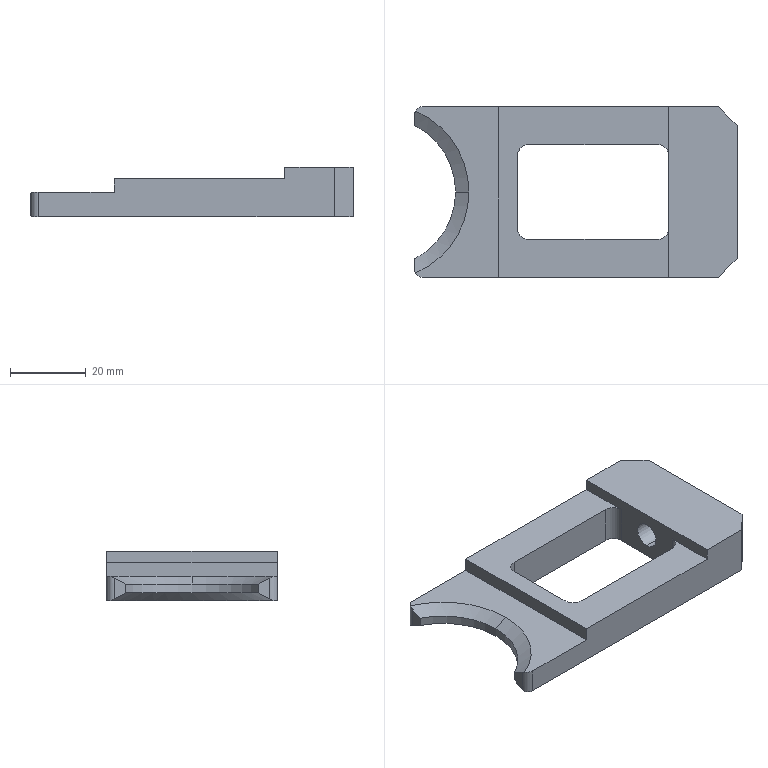Part | SolidWorks | features ICE 6, Chamfer 3, Fillet 3, Extrusion 1, HoleWzd 1 | 1 solid | 28 faces | box 85 x 45 x 13 mm | volume 24143 mm3 | plane 16 | cylinder 9 | cone 3 | commonest cylinder face diameters 6 x4 4 x2 6.8 x2 39.5 x1
STEP:
#1=CARTESIAN_POINT('',(80.,0.,-0.1));
#2=VERTEX_POINT('',#1);
#3=CARTESIAN_POINT('',(80.,0.,-6.9));
#4=VERTEX_POINT('',#3);
#5=CARTESIAN_POINT('',(80.,0.,-3.5));
#6=DIRECTION('',(1.,0.,0.));
#7=DIRECTION('',(0.,0.,-1.));
#8=AXIS2_PLACEMENT_3D('',#5,#6,#7);
#9=CIRCLE('',#8,3.4);
#10=EDGE_CURVE('',#2,#4,#9,.T.);
#11=ORIENTED_EDGE('',*,*,#10,.F.);
#12=CARTESIAN_POINT('',(98.,0.,-0.1));
#13=VERTEX_POINT('',#12);
#14=CARTESIAN_POINT('',(98.,0.,-0.1));
#15=DIRECTION('',(1.,0.,0.));
#16=VECTOR('',#15,1000.);
#17=LINE('',#14,#16);
#18=EDGE_CURVE('',#2,#13,#17,.T.);
#19=ORIENTED_EDGE('',*,*,#18,.T.);
#20=CARTESIAN_POINT('',(98.,0.,-6.9));
#21=VERTEX_POINT('',#20);
#22=CARTESIAN_POINT('',(98.,0.,-3.5));
#23=DIRECTION('',(1.,0.,0.));
#24=DIRECTION('',(0.,0.,-1.));
#25=AXIS2_PLACEMENT_3D('',#22,#23,#24);
#26=CIRCLE('',#25,3.4);
#27=EDGE_CURVE('',#13,#21,#26,.T.);
#28=ORIENTED_EDGE('',*,*,#27,.T.);
#29=CARTESIAN_POINT('',(98.,0.,-6.9));
#30=DIRECTION('',(1.,0.,0.));
#31=VECTOR('',#30,1000.);
#32=LINE('',#29,#31);
#33=EDGE_CURVE('',#4,#21,#32,.T.);
#34=ORIENTED_EDGE('',*,*,#33,.F.);
#35=EDGE_LOOP('',(#11,#19,#28,#34));
#36=FACE_OUTER_BOUND('',#35,.T.);
#37=CARTESIAN_POINT('',(98.,0.,-3.5));
#38=DIRECTION('',(1.,0.,0.));
#39=DIRECTION('',(0.,0.,-1.));
#40=AXIS2_PLACEMENT_3D('',#37,#38,#39);
#41=CYLINDRICAL_SURFACE('',#40,3.4);
#42=ADVANCED_FACE('',(#36),#41,.F.);
#43=CARTESIAN_POINT('',(23.75,0.,-5.62));
#44=VERTEX_POINT('',#43);
#45=CARTESIAN_POINT('',(13.,17.58,-5.62));
#46=VERTEX_POINT('',#45);
#47=CARTESIAN_POINT('',(4.,0.,-5.62));
#48=DIRECTION('',(0.,0.,1.));
#49=DIRECTION('',(-1.,0.,0.));
#50=AXIS2_PLACEMENT_3D('',#47,#48,#49);
#51=CIRCLE('',#50,19.75);
#52=EDGE_CURVE('',#44,#46,#51,.T.);
#53=ORIENTED_EDGE('',*,*,#52,.F.);
#54=CARTESIAN_POINT('',(27.25,0.,-3.6));
#55=VERTEX_POINT('',#54);
#56=CARTESIAN_POINT('',(23.75,0.,-5.62));
#57=DIRECTION('',(0.8661,0.,0.4999));
#58=VECTOR('',#57,1000.);
#59=LINE('',#56,#58);
#60=EDGE_CURVE('',#44,#55,#59,.T.);
#61=ORIENTED_EDGE('',*,*,#60,.T.);
#62=CARTESIAN_POINT('',(13.192,21.356,-3.6));
#63=VERTEX_POINT('',#62);
#64=CARTESIAN_POINT('',(4.,0.,-3.6));
#65=DIRECTION('',(0.,0.,-1.));
#66=DIRECTION('',(-1.,0.,0.));
#67=AXIS2_PLACEMENT_3D('',#64,#65,#66);
#68=CIRCLE('',#67,23.25);
#69=EDGE_CURVE('',#63,#55,#68,.T.);
#70=ORIENTED_EDGE('',*,*,#69,.F.);
#71=CARTESIAN_POINT('',(13.,20.5,-4.097));
#72=VERTEX_POINT('',#71);
#73=CARTESIAN_POINT('',(13.192,21.356,-3.6));
#74=CARTESIAN_POINT('',(13.065,21.088,-3.771));
#75=CARTESIAN_POINT('',(13.,20.803,-3.937));
#76=CARTESIAN_POINT('',(13.,20.5,-4.097));
#77=B_SPLINE_CURVE_WITH_KNOTS('',3,(#73,#74,#75,#76),.UNSPECIFIED.,.F.,.F.,(4,4),(0.,0.001008),.UNSPECIFIED.);
#78=EDGE_CURVE('',#63,#72,#77,.T.);
#79=ORIENTED_EDGE('',*,*,#78,.T.);
#80=CARTESIAN_POINT('',(13.,17.58,-5.62));
#81=CARTESIAN_POINT('',(13.,18.556,-5.119));
#82=CARTESIAN_POINT('',(13.,19.529,-4.61));
#83=CARTESIAN_POINT('',(13.,20.5,-4.097));
#84=B_SPLINE_CURVE_WITH_KNOTS('',3,(#80,#81,#82,#83),.UNSPECIFIED.,.F.,.F.,(4,4),(0.04213,0.04546),.UNSPECIFIED.);
#85=EDGE_CURVE('',#46,#72,#84,.T.);
#86=ORIENTED_EDGE('',*,*,#85,.F.);
#87=EDGE_LOOP('',(#53,#61,#70,#79,#86));
#88=FACE_OUTER_BOUND('',#87,.T.);
#89=CARTESIAN_POINT('',(4.,0.,-5.62));
#90=DIRECTION('',(0.,0.,1.));
#91=DIRECTION('',(1.,0.,0.));
#92=AXIS2_PLACEMENT_3D('',#89,#90,#91);
#93=CONICAL_SURFACE('',#92,19.75,1.047);
#94=ADVANCED_FACE('',(#88),#93,.F.);
#95=CARTESIAN_POINT('',(80.,-9.5,0.));
#96=VERTEX_POINT('',#95);
#97=CARTESIAN_POINT('',(80.,-22.5,0.));
#98=VERTEX_POINT('',#97);
#99=CARTESIAN_POINT('',(80.,22.5,0.));
#100=DIRECTION('',(0.,-1.,0.));
#101=VECTOR('',#100,1000.);
#102=LINE('',#99,#101);
#103=EDGE_CURVE('',#96,#98,#102,.T.);
#104=ORIENTED_EDGE('',*,*,#103,.F.);
#105=CARTESIAN_POINT('',(77.,-12.5,0.));
#106=VERTEX_POINT('',#105);
#107=CARTESIAN_POINT('',(77.,-9.5,0.));
#108=DIRECTION('',(0.,0.,-1.));
#109=DIRECTION('',(-1.,0.,0.));
#110=AXIS2_PLACEMENT_3D('',#107,#108,#109);
#111=CIRCLE('',#110,3.);
#112=EDGE_CURVE('',#96,#106,#111,.T.);
#113=ORIENTED_EDGE('',*,*,#112,.T.);
#114=CARTESIAN_POINT('',(43.,-12.5,0.));
#115=VERTEX_POINT('',#114);
#116=CARTESIAN_POINT('',(40.,-12.5,0.));
#117=DIRECTION('',(1.,0.,0.));
#118=VECTOR('',#117,1000.);
#119=LINE('',#116,#118);
#120=EDGE_CURVE('',#115,#106,#119,.T.);
#121=ORIENTED_EDGE('',*,*,#120,.F.);
#122=CARTESIAN_POINT('',(40.,-9.5,0.));
#123=VERTEX_POINT('',#122);
#124=CARTESIAN_POINT('',(43.,-9.5,0.));
#125=DIRECTION('',(0.,0.,-1.));
#126=DIRECTION('',(-1.,0.,0.));
#127=AXIS2_PLACEMENT_3D('',#124,#125,#126);
#128=CIRCLE('',#127,3.);
#129=EDGE_CURVE('',#115,#123,#128,.T.);
#130=ORIENTED_EDGE('',*,*,#129,.T.);
#131=CARTESIAN_POINT('',(40.,9.5,0.));
#132=VERTEX_POINT('',#131);
#133=CARTESIAN_POINT('',(40.,12.5,0.));
#134=DIRECTION('',(0.,-1.,0.));
#135=VECTOR('',#134,1000.);
#136=LINE('',#133,#135);
#137=EDGE_CURVE('',#132,#123,#136,.T.);
#138=ORIENTED_EDGE('',*,*,#137,.F.);
#139=CARTESIAN_POINT('',(43.,12.5,0.));
#140=VERTEX_POINT('',#139);
#141=CARTESIAN_POINT('',(43.,9.5,0.));
#142=DIRECTION('',(0.,0.,-1.));
#143=DIRECTION('',(-1.,0.,0.));
#144=AXIS2_PLACEMENT_3D('',#141,#142,#143);
#145=CIRCLE('',#144,3.);
#146=EDGE_CURVE('',#132,#140,#145,.T.);
#147=ORIENTED_EDGE('',*,*,#146,.T.);
#148=CARTESIAN_POINT('',(77.,12.5,0.));
#149=VERTEX_POINT('',#148);
#150=CARTESIAN_POINT('',(40.,12.5,0.));
#151=DIRECTION('',(-1.,0.,0.));
#152=VECTOR('',#151,1000.);
#153=LINE('',#150,#152);
#154=EDGE_CURVE('',#149,#140,#153,.T.);
#155=ORIENTED_EDGE('',*,*,#154,.F.);
#156=CARTESIAN_POINT('',(80.,9.5,0.));
#157=VERTEX_POINT('',#156);
#158=CARTESIAN_POINT('',(77.,9.5,0.));
#159=DIRECTION('',(0.,0.,-1.));
#160=DIRECTION('',(-1.,0.,0.));
#161=AXIS2_PLACEMENT_3D('',#158,#159,#160);
#162=CIRCLE('',#161,3.);
#163=EDGE_CURVE('',#149,#157,#162,.T.);
#164=ORIENTED_EDGE('',*,*,#163,.T.);
#165=CARTESIAN_POINT('',(80.,22.5,0.));
#166=VERTEX_POINT('',#165);
#167=CARTESIAN_POINT('',(80.,22.5,0.));
#168=DIRECTION('',(0.,-1.,0.));
#169=VECTOR('',#168,1000.);
#170=LINE('',#167,#169);
#171=EDGE_CURVE('',#166,#157,#170,.T.);
#172=ORIENTED_EDGE('',*,*,#171,.F.);
#173=CARTESIAN_POINT('',(35.,22.5,0.));
#174=VERTEX_POINT('',#173);
#175=CARTESIAN_POINT('',(0.,22.5,0.));
#176=DIRECTION('',(1.,0.,0.));
#177=VECTOR('',#176,1000.);
#178=LINE('',#175,#177);
#179=EDGE_CURVE('',#174,#166,#178,.T.);
#180=ORIENTED_EDGE('',*,*,#179,.F.);
#181=CARTESIAN_POINT('',(35.,-22.5,0.));
#182=VERTEX_POINT('',#181);
#183=CARTESIAN_POINT('',(35.,22.5,0.));
#184=DIRECTION('',(0.,-1.,0.));
#185=VECTOR('',#184,1000.);
#186=LINE('',#183,#185);
#187=EDGE_CURVE('',#174,#182,#186,.T.);
#188=ORIENTED_EDGE('',*,*,#187,.T.);
#189=CARTESIAN_POINT('',(0.,-22.5,0.));
#190=DIRECTION('',(1.,0.,0.));
#191=VECTOR('',#190,1000.);
#192=LINE('',#189,#191);
#193=EDGE_CURVE('',#182,#98,#192,.T.);
#194=ORIENTED_EDGE('',*,*,#193,.T.);
#195=EDGE_LOOP('',(#104,#113,#121,#130,#138,#147,#155,#164,#172,#180,#188,#194));
#196=FACE_OUTER_BOUND('',#195,.T.);
#197=CARTESIAN_POINT('',(0.,22.5,0.));
#198=DIRECTION('',(0.,0.,-1.));
#199=DIRECTION('',(-1.,0.,0.));
#200=AXIS2_PLACEMENT_3D('',#197,#198,#199);
#201=PLANE('',#200);
#202=ADVANCED_FACE('',(#196),#201,.F.);
#203=CARTESIAN_POINT('',(80.,0.,-3.5));
#204=DIRECTION('',(1.,0.,0.));
#205=DIRECTION('',(0.,0.,-1.));
#206=AXIS2_PLACEMENT_3D('',#203,#204,#205);
#207=CIRCLE('',#206,3.4);
#208=EDGE_CURVE('',#4,#2,#207,.T.);
#209=ORIENTED_EDGE('',*,*,#208,.T.);
#210=ORIENTED_EDGE('',*,*,#10,.T.);
#211=EDGE_LOOP('',(#209,#210));
#212=FACE_BOUND('',#211,.T.);
#213=ORIENTED_EDGE('',*,*,#171,.T.);
#214=CARTESIAN_POINT('',(80.,9.5,-10.));
#215=VERTEX_POINT('',#214);
#216=CARTESIAN_POINT('',(80.,9.5,-10.));
#217=DIRECTION('',(0.,0.,-1.));
#218=VECTOR('',#217,1000.);
#219=LINE('',#216,#218);
#220=EDGE_CURVE('',#157,#215,#219,.T.);
#221=ORIENTED_EDGE('',*,*,#220,.T.);
#222=CARTESIAN_POINT('',(80.,-9.5,-10.));
#223=VERTEX_POINT('',#222);
#224=CARTESIAN_POINT('',(80.,22.5,-10.));
#225=DIRECTION('',(0.,1.,0.));
#226=VECTOR('',#225,1000.);
#227=LINE('',#224,#226);
#228=EDGE_CURVE('',#223,#215,#227,.T.);
#229=ORIENTED_EDGE('',*,*,#228,.F.);
#230=CARTESIAN_POINT('',(80.,-9.5,0.));
#231=DIRECTION('',(0.,0.,1.));
#232=VECTOR('',#231,1000.);
#233=LINE('',#230,#232);
#234=EDGE_CURVE('',#223,#96,#233,.T.);
#235=ORIENTED_EDGE('',*,*,#234,.T.);
#236=ORIENTED_EDGE('',*,*,#103,.T.);
#237=CARTESIAN_POINT('',(80.,-22.5,3.));
#238=VERTEX_POINT('',#237);
#239=CARTESIAN_POINT('',(80.,-22.5,0.));
#240=DIRECTION('',(0.,0.,1.));
#241=VECTOR('',#240,1000.);
#242=LINE('',#239,#241);
#243=EDGE_CURVE('',#98,#238,#242,.T.);
#244=ORIENTED_EDGE('',*,*,#243,.T.);
#245=CARTESIAN_POINT('',(80.,22.5,3.));
#246=VERTEX_POINT('',#245);
#247=CARTESIAN_POINT('',(80.,22.5,3.));
#248=DIRECTION('',(0.,-1.,0.));
#249=VECTOR('',#248,1000.);
#250=LINE('',#247,#249);
#251=EDGE_CURVE('',#246,#238,#250,.T.);
#252=ORIENTED_EDGE('',*,*,#251,.F.);
#253=CARTESIAN_POINT('',(80.,22.5,0.));
#254=DIRECTION('',(0.,0.,1.));
#255=VECTOR('',#254,1000.);
#256=LINE('',#253,#255);
#257=EDGE_CURVE('',#166,#246,#256,.T.);
#258=ORIENTED_EDGE('',*,*,#257,.F.);
#259=EDGE_LOOP('',(#213,#221,#229,#235,#236,#244,#252,#258));
#260=FACE_OUTER_BOUND('',#259,.T.);
#261=CARTESIAN_POINT('',(80.,22.5,0.));
#262=DIRECTION('',(1.,0.,0.));
#263=DIRECTION('',(0.,0.,-1.));
#264=AXIS2_PLACEMENT_3D('',#261,#262,#263);
#265=PLANE('',#264);
#266=ADVANCED_FACE('',(#212,#260),#265,.F.);
#267=CARTESIAN_POINT('',(93.,-22.5,3.));
#268=VERTEX_POINT('',#267);
#269=CARTESIAN_POINT('',(80.,-22.5,3.));
#270=DIRECTION('',(1.,0.,0.));
#271=VECTOR('',#270,1000.);
#272=LINE('',#269,#271);
#273=EDGE_CURVE('',#238,#268,#272,.T.);
#274=ORIENTED_EDGE('',*,*,#273,.T.);
#275=CARTESIAN_POINT('',(98.,-17.5,3.));
#276=VERTEX_POINT('',#275);
#277=CARTESIAN_POINT('',(98.,-17.5,3.));
#278=DIRECTION('',(0.7071,0.7071,0.));
#279=VECTOR('',#278,1000.);
#280=LINE('',#277,#279);
#281=EDGE_CURVE('',#268,#276,#280,.T.);
#282=ORIENTED_EDGE('',*,*,#281,.T.);
#283=CARTESIAN_POINT('',(98.,17.5,3.));
#284=VERTEX_POINT('',#283);
#285=CARTESIAN_POINT('',(98.,22.5,3.));
#286=DIRECTION('',(0.,-1.,0.));
#287=VECTOR('',#286,1000.);
#288=LINE('',#285,#287);
#289=EDGE_CURVE('',#284,#276,#288,.T.);
#290=ORIENTED_EDGE('',*,*,#289,.F.);
#291=CARTESIAN_POINT('',(93.,22.5,3.));
#292=VERTEX_POINT('',#291);
#293=CARTESIAN_POINT('',(93.,22.5,3.));
#294=DIRECTION('',(-0.7071,0.7071,0.));
#295=VECTOR('',#294,1000.);
#296=LINE('',#293,#295);
#297=EDGE_CURVE('',#284,#292,#296,.T.);
#298=ORIENTED_EDGE('',*,*,#297,.T.);
#299=CARTESIAN_POINT('',(80.,22.5,3.));
#300=DIRECTION('',(1.,0.,0.));
#301=VECTOR('',#300,1000.);
#302=LINE('',#299,#301);
#303=EDGE_CURVE('',#246,#292,#302,.T.);
#304=ORIENTED_EDGE('',*,*,#303,.F.);
#305=ORIENTED_EDGE('',*,*,#251,.T.);
#306=EDGE_LOOP('',(#274,#282,#290,#298,#304,#305));
#307=FACE_OUTER_BOUND('',#306,.T.);
#308=CARTESIAN_POINT('',(80.,22.5,3.));
#309=DIRECTION('',(0.,0.,-1.));
#310=DIRECTION('',(-1.,0.,0.));
#311=AXIS2_PLACEMENT_3D('',#308,#309,#310);
#312=PLANE('',#311);
#313=ADVANCED_FACE('',(#307),#312,.F.);
#314=CARTESIAN_POINT('',(98.,0.,-3.5));
#315=DIRECTION('',(1.,0.,0.));
#316=DIRECTION('',(0.,0.,-1.));
#317=AXIS2_PLACEMENT_3D('',#314,#315,#316);
#318=CIRCLE('',#317,3.4);
#319=EDGE_CURVE('',#21,#13,#318,.T.);
#320=ORIENTED_EDGE('',*,*,#319,.F.);
#321=ORIENTED_EDGE('',*,*,#27,.F.);
#322=EDGE_LOOP('',(#320,#321));
#323=FACE_BOUND('',#322,.T.);
#324=ORIENTED_EDGE('',*,*,#289,.T.);
#325=CARTESIAN_POINT('',(98.,-17.5,-10.));
#326=VERTEX_POINT('',#325);
#327=CARTESIAN_POINT('',(98.,-17.5,3.));
#328=DIRECTION('',(0.,0.,-1.));
#329=VECTOR('',#328,1000.);
#330=LINE('',#327,#329);
#331=EDGE_CURVE('',#276,#326,#330,.T.);
#332=ORIENTED_EDGE('',*,*,#331,.T.);
#333=CARTESIAN_POINT('',(98.,17.5,-10.));
#334=VERTEX_POINT('',#333);
#335=CARTESIAN_POINT('',(98.,22.5,-10.));
#336=DIRECTION('',(0.,-1.,0.));
#337=VECTOR('',#336,1000.);
#338=LINE('',#335,#337);
#339=EDGE_CURVE('',#334,#326,#338,.T.);
#340=ORIENTED_EDGE('',*,*,#339,.F.);
#341=CARTESIAN_POINT('',(98.,17.5,3.));
#342=DIRECTION('',(0.,0.,1.));
#343=VECTOR('',#342,1000.);
#344=LINE('',#341,#343);
#345=EDGE_CURVE('',#334,#284,#344,.T.);
#346=ORIENTED_EDGE('',*,*,#345,.T.);
#347=EDGE_LOOP('',(#324,#332,#340,#346));
#348=FACE_OUTER_BOUND('',#347,.T.);
#349=CARTESIAN_POINT('',(98.,22.5,3.));
#350=DIRECTION('',(-1.,0.,0.));
#351=DIRECTION('',(0.,0.,1.));
#352=AXIS2_PLACEMENT_3D('',#349,#350,#351);
#353=PLANE('',#352);
#354=ADVANCED_FACE('',(#323,#348),#353,.F.);
#355=CARTESIAN_POINT('',(40.,9.5,-10.));
#356=VERTEX_POINT('',#355);
#357=CARTESIAN_POINT('',(40.,-9.5,-10.));
#358=VERTEX_POINT('',#357);
#359=CARTESIAN_POINT('',(40.,22.5,-10.));
#360=DIRECTION('',(0.,-1.,0.));
#361=VECTOR('',#360,1000.);
#362=LINE('',#359,#361);
#363=EDGE_CURVE('',#356,#358,#362,.T.);
#364=ORIENTED_EDGE('',*,*,#363,.T.);
#365=CARTESIAN_POINT('',(43.,-12.5,-10.));
#366=VERTEX_POINT('',#365);
#367=CARTESIAN_POINT('',(43.,-9.5,-10.));
#368=DIRECTION('',(0.,0.,1.));
#369=DIRECTION('',(1.,0.,0.));
#370=AXIS2_PLACEMENT_3D('',#367,#368,#369);
#371=CIRCLE('',#370,3.);
#372=EDGE_CURVE('',#358,#366,#371,.T.);
#373=ORIENTED_EDGE('',*,*,#372,.T.);
#374=CARTESIAN_POINT('',(77.,-12.5,-10.));
#375=VERTEX_POINT('',#374);
#376=CARTESIAN_POINT('',(98.,-12.5,-10.));
#377=DIRECTION('',(1.,0.,0.));
#378=VECTOR('',#377,1000.);
#379=LINE('',#376,#378);
#380=EDGE_CURVE('',#366,#375,#379,.T.);
#381=ORIENTED_EDGE('',*,*,#380,.T.);
#382=CARTESIAN_POINT('',(77.,-9.5,-10.));
#383=DIRECTION('',(0.,0.,1.));
#384=DIRECTION('',(1.,0.,0.));
#385=AXIS2_PLACEMENT_3D('',#382,#383,#384);
#386=CIRCLE('',#385,3.);
#387=EDGE_CURVE('',#375,#223,#386,.T.);
#388=ORIENTED_EDGE('',*,*,#387,.T.);
#389=ORIENTED_EDGE('',*,*,#228,.T.);
#390=CARTESIAN_POINT('',(77.,12.5,-10.));
#391=VERTEX_POINT('',#390);
#392=CARTESIAN_POINT('',(77.,9.5,-10.));
#393=DIRECTION('',(0.,0.,1.));
#394=DIRECTION('',(1.,0.,0.));
#395=AXIS2_PLACEMENT_3D('',#392,#393,#394);
#396=CIRCLE('',#395,3.);
#397=EDGE_CURVE('',#215,#391,#396,.T.);
#398=ORIENTED_EDGE('',*,*,#397,.T.);
#399=CARTESIAN_POINT('',(43.,12.5,-10.));
#400=VERTEX_POINT('',#399);
#401=CARTESIAN_POINT('',(98.,12.5,-10.));
#402=DIRECTION('',(-1.,0.,0.));
#403=VECTOR('',#402,1000.);
#404=LINE('',#401,#403);
#405=EDGE_CURVE('',#391,#400,#404,.T.);
#406=ORIENTED_EDGE('',*,*,#405,.T.);
#407=CARTESIAN_POINT('',(43.,9.5,-10.));
#408=DIRECTION('',(0.,0.,1.));
#409=DIRECTION('',(1.,0.,0.));
#410=AXIS2_PLACEMENT_3D('',#407,#408,#409);
#411=CIRCLE('',#410,3.);
#412=EDGE_CURVE('',#400,#356,#411,.T.);
#413=ORIENTED_EDGE('',*,*,#412,.T.);
#414=EDGE_LOOP('',(#364,#373,#381,#388,#389,#398,#406,#413));
#415=FACE_BOUND('',#414,.T.);
#416=CARTESIAN_POINT('',(13.192,-21.356,-10.));
#417=VERTEX_POINT('',#416);
#418=CARTESIAN_POINT('',(13.192,21.356,-10.));
#419=VERTEX_POINT('',#418);
#420=CARTESIAN_POINT('',(4.,0.,-10.));
#421=DIRECTION('',(0.,0.,1.));
#422=DIRECTION('',(1.,0.,0.));
#423=AXIS2_PLACEMENT_3D('',#420,#421,#422);
#424=CIRCLE('',#423,23.25);
#425=EDGE_CURVE('',#417,#419,#424,.T.);
#426=ORIENTED_EDGE('',*,*,#425,.T.);
#427=CARTESIAN_POINT('',(15.,22.5,-10.));
#428=VERTEX_POINT('',#427);
#429=CARTESIAN_POINT('',(15.,20.5,-10.));
#430=DIRECTION('',(0.,0.,-1.));
#431=DIRECTION('',(1.,0.,0.));
#432=AXIS2_PLACEMENT_3D('',#429,#430,#431);
#433=CIRCLE('',#432,2.);
#434=EDGE_CURVE('',#419,#428,#433,.T.);
#435=ORIENTED_EDGE('',*,*,#434,.T.);
#436=CARTESIAN_POINT('',(93.,22.5,-10.));
#437=VERTEX_POINT('',#436);
#438=CARTESIAN_POINT('',(98.,22.5,-10.));
#439=DIRECTION('',(-1.,0.,0.));
#440=VECTOR('',#439,1000.);
#441=LINE('',#438,#440);
#442=EDGE_CURVE('',#437,#428,#441,.T.);
#443=ORIENTED_EDGE('',*,*,#442,.F.);
#444=CARTESIAN_POINT('',(93.,22.5,-10.));
#445=DIRECTION('',(0.7071,-0.7071,0.));
#446=VECTOR('',#445,1000.);
#447=LINE('',#444,#446);
#448=EDGE_CURVE('',#437,#334,#447,.T.);
#449=ORIENTED_EDGE('',*,*,#448,.T.);
#450=ORIENTED_EDGE('',*,*,#339,.T.);
#451=CARTESIAN_POINT('',(93.,-22.5,-10.));
#452=VERTEX_POINT('',#451);
#453=CARTESIAN_POINT('',(98.,-17.5,-10.));
#454=DIRECTION('',(-0.7071,-0.7071,0.));
#455=VECTOR('',#454,1000.);
#456=LINE('',#453,#455);
#457=EDGE_CURVE('',#326,#452,#456,.T.);
#458=ORIENTED_EDGE('',*,*,#457,.T.);
#459=CARTESIAN_POINT('',(15.,-22.5,-10.));
#460=VERTEX_POINT('',#459);
#461=CARTESIAN_POINT('',(98.,-22.5,-10.));
#462=DIRECTION('',(-1.,0.,0.));
#463=VECTOR('',#462,1000.);
#464=LINE('',#461,#463);
#465=EDGE_CURVE('',#452,#460,#464,.T.);
#466=ORIENTED_EDGE('',*,*,#465,.T.);
#467=CARTESIAN_POINT('',(15.,-20.5,-10.));
#468=DIRECTION('',(0.,0.,-1.));
#469=DIRECTION('',(1.,0.,0.));
#470=AXIS2_PLACEMENT_3D('',#467,#468,#469);
#471=CIRCLE('',#470,2.);
#472=EDGE_CURVE('',#460,#417,#471,.T.);
#473=ORIENTED_EDGE('',*,*,#472,.T.);
#474=EDGE_LOOP('',(#426,#435,#443,#449,#450,#458,#466,#473));
#475=FACE_OUTER_BOUND('',#474,.T.);
#476=CARTESIAN_POINT('',(98.,22.5,-10.));
#477=DIRECTION('',(0.,0.,1.));
#478=DIRECTION('',(1.,0.,0.));
#479=AXIS2_PLACEMENT_3D('',#476,#477,#478);
#480=PLANE('',#479);
#481=ADVANCED_FACE('',(#415,#475),#480,.F.);
#482=ORIENTED_EDGE('',*,*,#442,.T.);
#483=CARTESIAN_POINT('',(15.,22.5,-3.6));
#484=VERTEX_POINT('',#483);
#485=CARTESIAN_POINT('',(15.,22.5,-3.6));
#486=DIRECTION('',(0.,0.,1.));
#487=VECTOR('',#486,1000.);
#488=LINE('',#485,#487);
#489=EDGE_CURVE('',#428,#484,#488,.T.);
#490=ORIENTED_EDGE('',*,*,#489,.T.);
#491=CARTESIAN_POINT('',(35.,22.5,-3.6));
#492=VERTEX_POINT('',#491);
#493=CARTESIAN_POINT('',(0.,22.5,-3.6));
#494=DIRECTION('',(1.,0.,0.));
#495=VECTOR('',#494,1000.);
#496=LINE('',#493,#495);
#497=EDGE_CURVE('',#484,#492,#496,.T.);
#498=ORIENTED_EDGE('',*,*,#497,.T.);
#499=CARTESIAN_POINT('',(35.,22.5,0.));
#500=DIRECTION('',(0.,0.,1.));
#501=VECTOR('',#500,1000.);
#502=LINE('',#499,#501);
#503=EDGE_CURVE('',#492,#174,#502,.T.);
#504=ORIENTED_EDGE('',*,*,#503,.T.);
#505=ORIENTED_EDGE('',*,*,#179,.T.);
#506=ORIENTED_EDGE('',*,*,#257,.T.);
#507=ORIENTED_EDGE('',*,*,#303,.T.);
#508=CARTESIAN_POINT('',(93.,22.5,-10.));
#509=DIRECTION('',(0.,0.,-1.));
#510=VECTOR('',#509,1000.);
#511=LINE('',#508,#510);
#512=EDGE_CURVE('',#292,#437,#511,.T.);
#513=ORIENTED_EDGE('',*,*,#512,.T.);
#514=EDGE_LOOP('',(#482,#490,#498,#504,#505,#506,#507,#513));
#515=FACE_OUTER_BOUND('',#514,.T.);
#516=CARTESIAN_POINT('',(0.,22.5,0.));
#517=DIRECTION('',(0.,1.,0.));
#518=DIRECTION('',(0.,0.,1.));
#519=AXIS2_PLACEMENT_3D('',#516,#517,#518);
#520=PLANE('',#519);
#521=ADVANCED_FACE('',(#515),#520,.T.);
#522=CARTESIAN_POINT('',(15.,-22.5,-3.6));
#523=VERTEX_POINT('',#522);
#524=CARTESIAN_POINT('',(35.,-22.5,-3.6));
#525=VERTEX_POINT('',#524);
#526=CARTESIAN_POINT('',(0.,-22.5,-3.6));
#527=DIRECTION('',(1.,0.,0.));
#528=VECTOR('',#527,1000.);
#529=LINE('',#526,#528);
#530=EDGE_CURVE('',#523,#525,#529,.T.);
#531=ORIENTED_EDGE('',*,*,#530,.F.);
#532=CARTESIAN_POINT('',(15.,-22.5,0.));
#533=DIRECTION('',(0.,0.,-1.));
#534=VECTOR('',#533,1000.);
#535=LINE('',#532,#534);
#536=EDGE_CURVE('',#523,#460,#535,.T.);
#537=ORIENTED_EDGE('',*,*,#536,.T.);
#538=ORIENTED_EDGE('',*,*,#465,.F.);
#539=CARTESIAN_POINT('',(93.,-22.5,0.));
#540=DIRECTION('',(0.,0.,1.));
#541=VECTOR('',#540,1000.);
#542=LINE('',#539,#541);
#543=EDGE_CURVE('',#452,#268,#542,.T.);
#544=ORIENTED_EDGE('',*,*,#543,.T.);
#545=ORIENTED_EDGE('',*,*,#273,.F.);
#546=ORIENTED_EDGE('',*,*,#243,.F.);
#547=ORIENTED_EDGE('',*,*,#193,.F.);
#548=CARTESIAN_POINT('',(35.,-22.5,0.));
#549=DIRECTION('',(0.,0.,1.));
#550=VECTOR('',#549,1000.);
#551=LINE('',#548,#550);
#552=EDGE_CURVE('',#525,#182,#551,.T.);
#553=ORIENTED_EDGE('',*,*,#552,.F.);
#554=EDGE_LOOP('',(#531,#537,#538,#544,#545,#546,#547,#553));
#555=FACE_OUTER_BOUND('',#554,.T.);
#556=CARTESIAN_POINT('',(0.,-22.5,0.));
#557=DIRECTION('',(0.,1.,0.));
#558=DIRECTION('',(0.,0.,1.));
#559=AXIS2_PLACEMENT_3D('',#556,#557,#558);
#560=PLANE('',#559);
#561=ADVANCED_FACE('',(#555),#560,.F.);
#562=ORIENTED_EDGE('',*,*,#281,.F.);
#563=ORIENTED_EDGE('',*,*,#543,.F.);
#564=ORIENTED_EDGE('',*,*,#457,.F.);
#565=ORIENTED_EDGE('',*,*,#331,.F.);
#566=EDGE_LOOP('',(#562,#563,#564,#565));
#567=FACE_OUTER_BOUND('',#566,.T.);
#568=CARTESIAN_POINT('',(98.,-17.5,3.));
#569=DIRECTION('',(-0.7071,0.7071,0.));
#570=DIRECTION('',(0.,0.,-1.));
#571=AXIS2_PLACEMENT_3D('',#568,#569,#570);
#572=PLANE('',#571);
#573=ADVANCED_FACE('',(#567),#572,.F.);
#574=ORIENTED_EDGE('',*,*,#297,.F.);
#575=ORIENTED_EDGE('',*,*,#345,.F.);
#576=ORIENTED_EDGE('',*,*,#448,.F.);
#577=ORIENTED_EDGE('',*,*,#512,.F.);
#578=EDGE_LOOP('',(#574,#575,#576,#577));
#579=FACE_OUTER_BOUND('',#578,.T.);
#580=CARTESIAN_POINT('',(93.,22.5,0.));
#581=DIRECTION('',(0.7071,0.7071,0.));
#582=DIRECTION('',(0.,0.,1.));
#583=AXIS2_PLACEMENT_3D('',#580,#581,#582);
#584=PLANE('',#583);
#585=ADVANCED_FACE('',(#579),#584,.T.);
#586=CARTESIAN_POINT('',(13.,17.58,-7.98));
#587=VERTEX_POINT('',#586);
#588=CARTESIAN_POINT('',(13.,-17.58,-7.98));
#589=VERTEX_POINT('',#588);
#590=CARTESIAN_POINT('',(4.,0.,-7.98));
#591=DIRECTION('',(0.,0.,-1.));
#592=DIRECTION('',(1.,0.,0.));
#593=AXIS2_PLACEMENT_3D('',#590,#591,#592);
#594=CIRCLE('',#593,19.75);
#595=EDGE_CURVE('',#587,#589,#594,.T.);
#596=ORIENTED_EDGE('',*,*,#595,.T.);
#597=CARTESIAN_POINT('',(13.,-17.58,-5.62));
#598=VERTEX_POINT('',#597);
#599=CARTESIAN_POINT('',(13.,-17.58,3.001));
#600=DIRECTION('',(0.,0.,1.));
#601=VECTOR('',#600,1000.);
#602=LINE('',#599,#601);
#603=EDGE_CURVE('',#589,#598,#602,.T.);
#604=ORIENTED_EDGE('',*,*,#603,.T.);
#605=CARTESIAN_POINT('',(4.,0.,-5.62));
#606=DIRECTION('',(0.,0.,1.));
#607=DIRECTION('',(-1.,0.,0.));
#608=AXIS2_PLACEMENT_3D('',#605,#606,#607);
#609=CIRCLE('',#608,19.75);
#610=EDGE_CURVE('',#598,#44,#609,.T.);
#611=ORIENTED_EDGE('',*,*,#610,.T.);
#612=ORIENTED_EDGE('',*,*,#52,.T.);
#613=CARTESIAN_POINT('',(13.,17.58,3.001));
#614=DIRECTION('',(0.,0.,-1.));
#615=VECTOR('',#614,1000.);
#616=LINE('',#613,#615);
#617=EDGE_CURVE('',#46,#587,#616,.T.);
#618=ORIENTED_EDGE('',*,*,#617,.T.);
#619=EDGE_LOOP('',(#596,#604,#611,#612,#618));
#620=FACE_OUTER_BOUND('',#619,.T.);
#621=CARTESIAN_POINT('',(4.,0.,3.001));
#622=DIRECTION('',(0.,0.,-1.));
#623=DIRECTION('',(-1.,0.,0.));
#624=AXIS2_PLACEMENT_3D('',#621,#622,#623);
#625=CYLINDRICAL_SURFACE('',#624,19.75);
#626=ADVANCED_FACE('',(#620),#625,.F.);
#627=ORIENTED_EDGE('',*,*,#497,.F.);
#628=CARTESIAN_POINT('',(15.,20.5,-3.6));
#629=DIRECTION('',(0.,0.,1.));
#630=DIRECTION('',(-1.,0.,0.));
#631=AXIS2_PLACEMENT_3D('',#628,#629,#630);
#632=CIRCLE('',#631,2.);
#633=EDGE_CURVE('',#484,#63,#632,.T.);
#634=ORIENTED_EDGE('',*,*,#633,.T.);
#635=ORIENTED_EDGE('',*,*,#69,.T.);
#636=CARTESIAN_POINT('',(13.192,-21.356,-3.6));
#637=VERTEX_POINT('',#636);
#638=CARTESIAN_POINT('',(4.,0.,-3.6));
#639=DIRECTION('',(0.,0.,-1.));
#640=DIRECTION('',(-1.,0.,0.));
#641=AXIS2_PLACEMENT_3D('',#638,#639,#640);
#642=CIRCLE('',#641,23.25);
#643=EDGE_CURVE('',#55,#637,#642,.T.);
#644=ORIENTED_EDGE('',*,*,#643,.T.);
#645=CARTESIAN_POINT('',(15.,-20.5,-3.6));
#646=DIRECTION('',(0.,0.,1.));
#647=DIRECTION('',(-1.,0.,0.));
#648=AXIS2_PLACEMENT_3D('',#645,#646,#647);
#649=CIRCLE('',#648,2.);
#650=EDGE_CURVE('',#637,#523,#649,.T.);
#651=ORIENTED_EDGE('',*,*,#650,.T.);
#652=ORIENTED_EDGE('',*,*,#530,.T.);
#653=CARTESIAN_POINT('',(35.,22.5,-3.6));
#654=DIRECTION('',(0.,-1.,0.));
#655=VECTOR('',#654,1000.);
#656=LINE('',#653,#655);
#657=EDGE_CURVE('',#492,#525,#656,.T.);
#658=ORIENTED_EDGE('',*,*,#657,.F.);
#659=EDGE_LOOP('',(#627,#634,#635,#644,#651,#652,#658));
#660=FACE_OUTER_BOUND('',#659,.T.);
#661=CARTESIAN_POINT('',(0.,22.5,-3.6));
#662=DIRECTION('',(0.,0.,-1.));
#663=DIRECTION('',(-1.,0.,0.));
#664=AXIS2_PLACEMENT_3D('',#661,#662,#663);
#665=PLANE('',#664);
#666=ADVANCED_FACE('',(#660),#665,.F.);
#667=ORIENTED_EDGE('',*,*,#552,.T.);
#668=ORIENTED_EDGE('',*,*,#187,.F.);
#669=ORIENTED_EDGE('',*,*,#503,.F.);
#670=ORIENTED_EDGE('',*,*,#657,.T.);
#671=EDGE_LOOP('',(#667,#668,#669,#670));
#672=FACE_OUTER_BOUND('',#671,.T.);
#673=CARTESIAN_POINT('',(35.,22.5,0.));
#674=DIRECTION('',(1.,0.,0.));
#675=DIRECTION('',(0.,0.,-1.));
#676=AXIS2_PLACEMENT_3D('',#673,#674,#675);
#677=PLANE('',#676);
#678=ADVANCED_FACE('',(#672),#677,.F.);
#679=CARTESIAN_POINT('',(13.,20.5,-9.503));
#680=VERTEX_POINT('',#679);
#681=CARTESIAN_POINT('',(13.,20.5,-9.503));
#682=CARTESIAN_POINT('',(13.,19.529,-8.99));
#683=CARTESIAN_POINT('',(13.,18.556,-8.482));
#684=CARTESIAN_POINT('',(13.,17.58,-7.98));
#685=B_SPLINE_CURVE_WITH_KNOTS('',3,(#681,#682,#683,#684),.UNSPECIFIED.,.F.,.F.,(4,4),(0.001981,0.005274),.UNSPECIFIED.);
#686=EDGE_CURVE('',#680,#587,#685,.T.);
#687=ORIENTED_EDGE('',*,*,#686,.F.);
#688=CARTESIAN_POINT('',(13.,20.5,-9.503));
#689=CARTESIAN_POINT('',(13.,20.803,-9.663));
#690=CARTESIAN_POINT('',(13.065,21.088,-9.829));
#691=CARTESIAN_POINT('',(13.192,21.356,-10.));
#692=B_SPLINE_CURVE_WITH_KNOTS('',3,(#688,#689,#690,#691),.UNSPECIFIED.,.F.,.F.,(4,4),(0.,0.001008),.UNSPECIFIED.);
#693=EDGE_CURVE('',#680,#419,#692,.T.);
#694=ORIENTED_EDGE('',*,*,#693,.T.);
#695=ORIENTED_EDGE('',*,*,#425,.F.);
#696=CARTESIAN_POINT('',(13.,-20.5,-9.503));
#697=VERTEX_POINT('',#696);
#698=CARTESIAN_POINT('',(13.192,-21.356,-10.));
#699=CARTESIAN_POINT('',(13.065,-21.088,-9.829));
#700=CARTESIAN_POINT('',(13.,-20.803,-9.663));
#701=CARTESIAN_POINT('',(13.,-20.5,-9.503));
#702=B_SPLINE_CURVE_WITH_KNOTS('',3,(#698,#699,#700,#701),.UNSPECIFIED.,.F.,.F.,(4,4),(0.,0.001008),.UNSPECIFIED.);
#703=EDGE_CURVE('',#417,#697,#702,.T.);
#704=ORIENTED_EDGE('',*,*,#703,.T.);
#705=CARTESIAN_POINT('',(13.,-17.58,-7.98));
#706=CARTESIAN_POINT('',(13.,-18.556,-8.481));
#707=CARTESIAN_POINT('',(13.,-19.529,-8.99));
#708=CARTESIAN_POINT('',(13.,-20.5,-9.503));
#709=B_SPLINE_CURVE_WITH_KNOTS('',3,(#705,#706,#707,#708),.UNSPECIFIED.,.F.,.F.,(4,4),(0.04309,0.04643),.UNSPECIFIED.);
#710=EDGE_CURVE('',#589,#697,#709,.T.);
#711=ORIENTED_EDGE('',*,*,#710,.F.);
#712=ORIENTED_EDGE('',*,*,#595,.F.);
#713=EDGE_LOOP('',(#687,#694,#695,#704,#711,#712));
#714=FACE_OUTER_BOUND('',#713,.T.);
#715=CARTESIAN_POINT('',(4.,0.,-7.98));
#716=DIRECTION('',(0.,0.,-1.));
#717=DIRECTION('',(-1.,0.,0.));
#718=AXIS2_PLACEMENT_3D('',#715,#716,#717);
#719=CONICAL_SURFACE('',#718,19.75,1.047);
#720=ADVANCED_FACE('',(#714),#719,.F.);
#721=ORIENTED_EDGE('',*,*,#60,.F.);
#722=ORIENTED_EDGE('',*,*,#610,.F.);
#723=CARTESIAN_POINT('',(13.,-20.5,-4.097));
#724=VERTEX_POINT('',#723);
#725=CARTESIAN_POINT('',(13.,-20.5,-4.097));
#726=CARTESIAN_POINT('',(13.,-19.529,-4.61));
#727=CARTESIAN_POINT('',(13.,-18.556,-5.118));
#728=CARTESIAN_POINT('',(13.,-17.58,-5.62));
#729=B_SPLINE_CURVE_WITH_KNOTS('',3,(#725,#726,#727,#728),.UNSPECIFIED.,.F.,.F.,(4,4),(0.001062,0.004354),.UNSPECIFIED.);
#730=EDGE_CURVE('',#724,#598,#729,.T.);
#731=ORIENTED_EDGE('',*,*,#730,.F.);
#732=CARTESIAN_POINT('',(13.,-20.5,-4.097));
#733=CARTESIAN_POINT('',(13.,-20.803,-3.937));
#734=CARTESIAN_POINT('',(13.065,-21.088,-3.771));
#735=CARTESIAN_POINT('',(13.192,-21.356,-3.6));
#736=B_SPLINE_CURVE_WITH_KNOTS('',3,(#732,#733,#734,#735),.UNSPECIFIED.,.F.,.F.,(4,4),(0.,0.001008),.UNSPECIFIED.);
#737=EDGE_CURVE('',#724,#637,#736,.T.);
#738=ORIENTED_EDGE('',*,*,#737,.T.);
#739=ORIENTED_EDGE('',*,*,#643,.F.);
#740=EDGE_LOOP('',(#721,#722,#731,#738,#739));
#741=FACE_OUTER_BOUND('',#740,.T.);
#742=CARTESIAN_POINT('',(4.,0.,-5.62));
#743=DIRECTION('',(0.,0.,1.));
#744=DIRECTION('',(1.,0.,0.));
#745=AXIS2_PLACEMENT_3D('',#742,#743,#744);
#746=CONICAL_SURFACE('',#745,19.75,1.047);
#747=ADVANCED_FACE('',(#741),#746,.F.);
#748=ORIENTED_EDGE('',*,*,#380,.F.);
#749=CARTESIAN_POINT('',(43.,-12.5,0.));
#750=DIRECTION('',(0.,0.,1.));
#751=VECTOR('',#750,1000.);
#752=LINE('',#749,#751);
#753=EDGE_CURVE('',#366,#115,#752,.T.);
#754=ORIENTED_EDGE('',*,*,#753,.T.);
#755=ORIENTED_EDGE('',*,*,#120,.T.);
#756=CARTESIAN_POINT('',(77.,-12.5,-10.));
#757=DIRECTION('',(0.,0.,-1.));
#758=VECTOR('',#757,1000.);
#759=LINE('',#756,#758);
#760=EDGE_CURVE('',#106,#375,#759,.T.);
#761=ORIENTED_EDGE('',*,*,#760,.T.);
#762=EDGE_LOOP('',(#748,#754,#755,#761));
#763=FACE_OUTER_BOUND('',#762,.T.);
#764=CARTESIAN_POINT('',(40.,-12.5,-10.433));
#765=DIRECTION('',(0.,-1.,0.));
#766=DIRECTION('',(0.,0.,-1.));
#767=AXIS2_PLACEMENT_3D('',#764,#765,#766);
#768=PLANE('',#767);
#769=ADVANCED_FACE('',(#763),#768,.F.);
#770=ORIENTED_EDGE('',*,*,#137,.T.);
#771=CARTESIAN_POINT('',(40.,-9.5,-10.));
#772=DIRECTION('',(0.,0.,-1.));
#773=VECTOR('',#772,1000.);
#774=LINE('',#771,#773);
#775=EDGE_CURVE('',#123,#358,#774,.T.);
#776=ORIENTED_EDGE('',*,*,#775,.T.);
#777=ORIENTED_EDGE('',*,*,#363,.F.);
#778=CARTESIAN_POINT('',(40.,9.5,0.));
#779=DIRECTION('',(0.,0.,1.));
#780=VECTOR('',#779,1000.);
#781=LINE('',#778,#780);
#782=EDGE_CURVE('',#356,#132,#781,.T.);
#783=ORIENTED_EDGE('',*,*,#782,.T.);
#784=EDGE_LOOP('',(#770,#776,#777,#783));
#785=FACE_OUTER_BOUND('',#784,.T.);
#786=CARTESIAN_POINT('',(40.,12.5,-10.433));
#787=DIRECTION('',(-1.,0.,0.));
#788=DIRECTION('',(0.,0.,1.));
#789=AXIS2_PLACEMENT_3D('',#786,#787,#788);
#790=PLANE('',#789);
#791=ADVANCED_FACE('',(#785),#790,.F.);
#792=ORIENTED_EDGE('',*,*,#405,.F.);
#793=CARTESIAN_POINT('',(77.,12.5,0.));
#794=DIRECTION('',(0.,0.,1.));
#795=VECTOR('',#794,1000.);
#796=LINE('',#793,#795);
#797=EDGE_CURVE('',#391,#149,#796,.T.);
#798=ORIENTED_EDGE('',*,*,#797,.T.);
#799=ORIENTED_EDGE('',*,*,#154,.T.);
#800=CARTESIAN_POINT('',(43.,12.5,-10.));
#801=DIRECTION('',(0.,0.,-1.));
#802=VECTOR('',#801,1000.);
#803=LINE('',#800,#802);
#804=EDGE_CURVE('',#140,#400,#803,.T.);
#805=ORIENTED_EDGE('',*,*,#804,.T.);
#806=EDGE_LOOP('',(#792,#798,#799,#805));
#807=FACE_OUTER_BOUND('',#806,.T.);
#808=CARTESIAN_POINT('',(40.,12.5,-10.433));
#809=DIRECTION('',(0.,1.,0.));
#810=DIRECTION('',(0.,0.,1.));
#811=AXIS2_PLACEMENT_3D('',#808,#809,#810);
#812=PLANE('',#811);
#813=ADVANCED_FACE('',(#807),#812,.F.);
#814=ORIENTED_EDGE('',*,*,#372,.F.);
#815=ORIENTED_EDGE('',*,*,#775,.F.);
#816=ORIENTED_EDGE('',*,*,#129,.F.);
#817=ORIENTED_EDGE('',*,*,#753,.F.);
#818=EDGE_LOOP('',(#814,#815,#816,#817));
#819=FACE_OUTER_BOUND('',#818,.T.);
#820=CARTESIAN_POINT('',(43.,-9.5,-10.433));
#821=DIRECTION('',(0.,0.,-1.));
#822=DIRECTION('',(-1.,0.,0.));
#823=AXIS2_PLACEMENT_3D('',#820,#821,#822);
#824=CYLINDRICAL_SURFACE('',#823,3.);
#825=ADVANCED_FACE('',(#819),#824,.F.);
#826=ORIENTED_EDGE('',*,*,#397,.F.);
#827=ORIENTED_EDGE('',*,*,#220,.F.);
#828=ORIENTED_EDGE('',*,*,#163,.F.);
#829=ORIENTED_EDGE('',*,*,#797,.F.);
#830=EDGE_LOOP('',(#826,#827,#828,#829));
#831=FACE_OUTER_BOUND('',#830,.T.);
#832=CARTESIAN_POINT('',(77.,9.5,-10.433));
#833=DIRECTION('',(0.,0.,-1.));
#834=DIRECTION('',(-1.,0.,0.));
#835=AXIS2_PLACEMENT_3D('',#832,#833,#834);
#836=CYLINDRICAL_SURFACE('',#835,3.);
#837=ADVANCED_FACE('',(#831),#836,.F.);
#838=ORIENTED_EDGE('',*,*,#387,.F.);
#839=ORIENTED_EDGE('',*,*,#760,.F.);
#840=ORIENTED_EDGE('',*,*,#112,.F.);
#841=ORIENTED_EDGE('',*,*,#234,.F.);
#842=EDGE_LOOP('',(#838,#839,#840,#841));
#843=FACE_OUTER_BOUND('',#842,.T.);
#844=CARTESIAN_POINT('',(77.,-9.5,0.));
#845=DIRECTION('',(0.,0.,-1.));
#846=DIRECTION('',(-1.,0.,0.));
#847=AXIS2_PLACEMENT_3D('',#844,#845,#846);
#848=CYLINDRICAL_SURFACE('',#847,3.);
#849=ADVANCED_FACE('',(#843),#848,.F.);
#850=ORIENTED_EDGE('',*,*,#412,.F.);
#851=ORIENTED_EDGE('',*,*,#804,.F.);
#852=ORIENTED_EDGE('',*,*,#146,.F.);
#853=ORIENTED_EDGE('',*,*,#782,.F.);
#854=EDGE_LOOP('',(#850,#851,#852,#853));
#855=FACE_OUTER_BOUND('',#854,.T.);
#856=CARTESIAN_POINT('',(43.,9.5,-10.433));
#857=DIRECTION('',(0.,0.,-1.));
#858=DIRECTION('',(-1.,0.,0.));
#859=AXIS2_PLACEMENT_3D('',#856,#857,#858);
#860=CYLINDRICAL_SURFACE('',#859,3.);
#861=ADVANCED_FACE('',(#855),#860,.F.);
#862=ORIENTED_EDGE('',*,*,#85,.T.);
#863=CARTESIAN_POINT('',(13.,20.5,-10.));
#864=DIRECTION('',(0.,0.,-1.));
#865=VECTOR('',#864,1000.);
#866=LINE('',#863,#865);
#867=EDGE_CURVE('',#72,#680,#866,.T.);
#868=ORIENTED_EDGE('',*,*,#867,.T.);
#869=ORIENTED_EDGE('',*,*,#686,.T.);
#870=ORIENTED_EDGE('',*,*,#617,.F.);
#871=EDGE_LOOP('',(#862,#868,#869,#870));
#872=FACE_OUTER_BOUND('',#871,.T.);
#873=CARTESIAN_POINT('',(13.,31.535,-10.433));
#874=DIRECTION('',(1.,0.,0.));
#875=DIRECTION('',(0.,1.,0.));
#876=AXIS2_PLACEMENT_3D('',#873,#874,#875);
#877=PLANE('',#876);
#878=ADVANCED_FACE('',(#872),#877,.F.);
#879=ORIENTED_EDGE('',*,*,#710,.T.);
#880=CARTESIAN_POINT('',(13.,-20.5,-10.433));
#881=DIRECTION('',(0.,0.,1.));
#882=VECTOR('',#881,1000.);
#883=LINE('',#880,#882);
#884=EDGE_CURVE('',#697,#724,#883,.T.);
#885=ORIENTED_EDGE('',*,*,#884,.T.);
#886=ORIENTED_EDGE('',*,*,#730,.T.);
#887=ORIENTED_EDGE('',*,*,#603,.F.);
#888=EDGE_LOOP('',(#879,#885,#886,#887));
#889=FACE_OUTER_BOUND('',#888,.T.);
#890=CARTESIAN_POINT('',(13.,31.535,-10.433));
#891=DIRECTION('',(1.,0.,0.));
#892=DIRECTION('',(0.,1.,0.));
#893=AXIS2_PLACEMENT_3D('',#890,#891,#892);
#894=PLANE('',#893);
#895=ADVANCED_FACE('',(#889),#894,.F.);
#896=ORIENTED_EDGE('',*,*,#633,.F.);
#897=ORIENTED_EDGE('',*,*,#489,.F.);
#898=ORIENTED_EDGE('',*,*,#434,.F.);
#899=ORIENTED_EDGE('',*,*,#693,.F.);
#900=ORIENTED_EDGE('',*,*,#867,.F.);
#901=ORIENTED_EDGE('',*,*,#78,.F.);
#902=EDGE_LOOP('',(#896,#897,#898,#899,#900,#901));
#903=FACE_OUTER_BOUND('',#902,.T.);
#904=CARTESIAN_POINT('',(15.,20.5,-10.433));
#905=DIRECTION('',(0.,0.,1.));
#906=DIRECTION('',(1.,0.,0.));
#907=AXIS2_PLACEMENT_3D('',#904,#905,#906);
#908=CYLINDRICAL_SURFACE('',#907,2.);
#909=ADVANCED_FACE('',(#903),#908,.T.);
#910=ORIENTED_EDGE('',*,*,#737,.F.);
#911=ORIENTED_EDGE('',*,*,#884,.F.);
#912=ORIENTED_EDGE('',*,*,#703,.F.);
#913=ORIENTED_EDGE('',*,*,#472,.F.);
#914=ORIENTED_EDGE('',*,*,#536,.F.);
#915=ORIENTED_EDGE('',*,*,#650,.F.);
#916=EDGE_LOOP('',(#910,#911,#912,#913,#914,#915));
#917=FACE_OUTER_BOUND('',#916,.T.);
#918=CARTESIAN_POINT('',(15.,-20.5,0.));
#919=DIRECTION('',(0.,0.,-1.));
#920=DIRECTION('',(-1.,0.,0.));
#921=AXIS2_PLACEMENT_3D('',#918,#919,#920);
#922=CYLINDRICAL_SURFACE('',#921,2.);
#923=ADVANCED_FACE('',(#917),#922,.T.);
#924=ORIENTED_EDGE('',*,*,#18,.F.);
#925=ORIENTED_EDGE('',*,*,#208,.F.);
#926=ORIENTED_EDGE('',*,*,#33,.T.);
#927=ORIENTED_EDGE('',*,*,#319,.T.);
#928=EDGE_LOOP('',(#924,#925,#926,#927));
#929=FACE_OUTER_BOUND('',#928,.T.);
#930=CARTESIAN_POINT('',(98.,0.,-3.5));
#931=DIRECTION('',(1.,0.,0.));
#932=DIRECTION('',(0.,0.,-1.));
#933=AXIS2_PLACEMENT_3D('',#930,#931,#932);
#934=CYLINDRICAL_SURFACE('',#933,3.4);
#935=ADVANCED_FACE('',(#929),#934,.F.);
#936=CLOSED_SHELL('',(#42,#94,#202,#266,#313,#354,#481,#521,#561,#573,#585,#626,#666,#678,#720,#747,#769,#791,#813,#825,#837,#849,#861,#878,#895,#909,#923,#935));
#937=MANIFOLD_SOLID_BREP('',#936);
#938=CARTESIAN_POINT('',(0.,0.,0.));
#939=DIRECTION('',(0.,0.,1.));
#940=DIRECTION('',(1.,0.,0.));
#941=AXIS2_PLACEMENT_3D('',#938,#939,#940);
#942=(LENGTH_UNIT()NAMED_UNIT(*)SI_UNIT(.MILLI.,.METRE.));
#943=UNCERTAINTY_MEASURE_WITH_UNIT(LENGTH_MEASURE(0.00001),#942,'','');
#944=(NAMED_UNIT(*)PLANE_ANGLE_UNIT()SI_UNIT($,.RADIAN.));
#945=(NAMED_UNIT(*)SI_UNIT($,.STERADIAN.)SOLID_ANGLE_UNIT());
#946=(GEOMETRIC_REPRESENTATION_CONTEXT(3)GLOBAL_UNCERTAINTY_ASSIGNED_CONTEXT((#943))GLOBAL_UNIT_ASSIGNED_CONTEXT((#942,#944,#945))REPRESENTATION_CONTEXT('',''));
#947=ADVANCED_BREP_SHAPE_REPRESENTATION('',(#937,#941),#946);